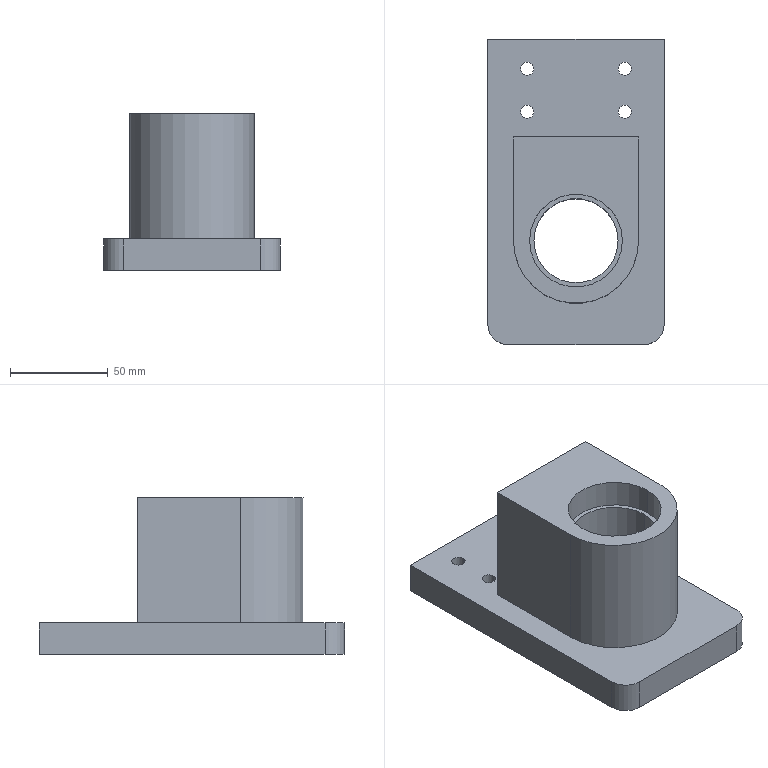Part | NX | 1 solid | 29 faces | box 90 x 156 x 80 mm | volume 416529 mm3 | cylinder 17 | plane 12 | commonest cylinder face diameters 6.8 x8 47.5 x4 20 x2 43 x2 64 x1
STEP:
#1=CARTESIAN_POINT('',(80.,0.,16.));
#2=VERTEX_POINT('',#1);
#3=CARTESIAN_POINT('',(90.,10.,16.));
#4=VERTEX_POINT('',#3);
#5=CARTESIAN_POINT('',(80.,10.,16.));
#6=DIRECTION('',(0.,0.,1.));
#7=DIRECTION('',(-1.,0.,0.));
#8=AXIS2_PLACEMENT_3D('',#5,#6,#7);
#9=CIRCLE('',#8,10.);
#10=EDGE_CURVE('',#2,#4,#9,.T.);
#11=ORIENTED_EDGE('',*,*,#10,.F.);
#12=CARTESIAN_POINT('',(80.,0.,0.));
#13=VERTEX_POINT('',#12);
#14=CARTESIAN_POINT('',(80.,0.,16.));
#15=DIRECTION('',(0.,0.,1.));
#16=VECTOR('',#15,1000.);
#17=LINE('',#14,#16);
#18=EDGE_CURVE('',#13,#2,#17,.T.);
#19=ORIENTED_EDGE('',*,*,#18,.F.);
#20=CARTESIAN_POINT('',(90.,10.,0.));
#21=VERTEX_POINT('',#20);
#22=CARTESIAN_POINT('',(80.,10.,0.));
#23=DIRECTION('',(0.,0.,-1.));
#24=DIRECTION('',(-1.,0.,0.));
#25=AXIS2_PLACEMENT_3D('',#22,#23,#24);
#26=CIRCLE('',#25,10.);
#27=EDGE_CURVE('',#21,#13,#26,.T.);
#28=ORIENTED_EDGE('',*,*,#27,.F.);
#29=CARTESIAN_POINT('',(90.,10.,16.));
#30=DIRECTION('',(0.,0.,-1.));
#31=VECTOR('',#30,1000.);
#32=LINE('',#29,#31);
#33=EDGE_CURVE('',#4,#21,#32,.T.);
#34=ORIENTED_EDGE('',*,*,#33,.F.);
#35=EDGE_LOOP('',(#11,#19,#28,#34));
#36=FACE_BOUND('',#35,.T.);
#37=CARTESIAN_POINT('',(80.,10.,16.));
#38=DIRECTION('',(0.,0.,-1.));
#39=DIRECTION('',(-1.,0.,0.));
#40=AXIS2_PLACEMENT_3D('',#37,#38,#39);
#41=CYLINDRICAL_SURFACE('',#40,10.);
#42=ADVANCED_FACE('',(#36),#41,.T.);
#43=CARTESIAN_POINT('',(0.,10.,16.));
#44=VERTEX_POINT('',#43);
#45=CARTESIAN_POINT('',(10.,0.,16.));
#46=VERTEX_POINT('',#45);
#47=CARTESIAN_POINT('',(10.,10.,16.));
#48=DIRECTION('',(0.,0.,1.));
#49=DIRECTION('',(-1.,0.,0.));
#50=AXIS2_PLACEMENT_3D('',#47,#48,#49);
#51=CIRCLE('',#50,10.);
#52=EDGE_CURVE('',#44,#46,#51,.T.);
#53=ORIENTED_EDGE('',*,*,#52,.F.);
#54=CARTESIAN_POINT('',(0.,10.,0.));
#55=VERTEX_POINT('',#54);
#56=CARTESIAN_POINT('',(0.,10.,16.));
#57=DIRECTION('',(0.,0.,1.));
#58=VECTOR('',#57,1000.);
#59=LINE('',#56,#58);
#60=EDGE_CURVE('',#55,#44,#59,.T.);
#61=ORIENTED_EDGE('',*,*,#60,.F.);
#62=CARTESIAN_POINT('',(10.,0.,0.));
#63=VERTEX_POINT('',#62);
#64=CARTESIAN_POINT('',(10.,10.,0.));
#65=DIRECTION('',(0.,0.,-1.));
#66=DIRECTION('',(-1.,0.,0.));
#67=AXIS2_PLACEMENT_3D('',#64,#65,#66);
#68=CIRCLE('',#67,10.);
#69=EDGE_CURVE('',#63,#55,#68,.T.);
#70=ORIENTED_EDGE('',*,*,#69,.F.);
#71=CARTESIAN_POINT('',(10.,0.,16.));
#72=DIRECTION('',(0.,0.,-1.));
#73=VECTOR('',#72,1000.);
#74=LINE('',#71,#73);
#75=EDGE_CURVE('',#46,#63,#74,.T.);
#76=ORIENTED_EDGE('',*,*,#75,.F.);
#77=EDGE_LOOP('',(#53,#61,#70,#76));
#78=FACE_BOUND('',#77,.T.);
#79=CARTESIAN_POINT('',(10.,10.,16.));
#80=DIRECTION('',(0.,0.,-1.));
#81=DIRECTION('',(-1.,0.,0.));
#82=AXIS2_PLACEMENT_3D('',#79,#80,#81);
#83=CYLINDRICAL_SURFACE('',#82,10.);
#84=ADVANCED_FACE('',(#78),#83,.T.);
#85=CARTESIAN_POINT('',(73.4,141.,16.));
#86=VERTEX_POINT('',#85);
#87=CARTESIAN_POINT('',(73.4,141.,0.));
#88=VERTEX_POINT('',#87);
#89=CARTESIAN_POINT('',(73.4,141.,0.));
#90=DIRECTION('',(0.,0.,-1.));
#91=VECTOR('',#90,1000.);
#92=LINE('',#89,#91);
#93=EDGE_CURVE('',#86,#88,#92,.T.);
#94=ORIENTED_EDGE('',*,*,#93,.F.);
#95=CARTESIAN_POINT('',(66.6,141.,16.));
#96=VERTEX_POINT('',#95);
#97=CARTESIAN_POINT('',(70.,141.,16.));
#98=DIRECTION('',(0.,0.,-1.));
#99=DIRECTION('',(-1.,0.,0.));
#100=AXIS2_PLACEMENT_3D('',#97,#98,#99);
#101=CIRCLE('',#100,3.4);
#102=EDGE_CURVE('',#96,#86,#101,.T.);
#103=ORIENTED_EDGE('',*,*,#102,.F.);
#104=CARTESIAN_POINT('',(66.6,141.,0.));
#105=VERTEX_POINT('',#104);
#106=CARTESIAN_POINT('',(66.6,141.,0.));
#107=DIRECTION('',(0.,0.,-1.));
#108=VECTOR('',#107,1000.);
#109=LINE('',#106,#108);
#110=EDGE_CURVE('',#96,#105,#109,.T.);
#111=ORIENTED_EDGE('',*,*,#110,.T.);
#112=CARTESIAN_POINT('',(70.,141.,0.));
#113=DIRECTION('',(0.,0.,-1.));
#114=DIRECTION('',(-1.,0.,0.));
#115=AXIS2_PLACEMENT_3D('',#112,#113,#114);
#116=CIRCLE('',#115,3.4);
#117=EDGE_CURVE('',#105,#88,#116,.T.);
#118=ORIENTED_EDGE('',*,*,#117,.T.);
#119=EDGE_LOOP('',(#94,#103,#111,#118));
#120=FACE_BOUND('',#119,.T.);
#121=CARTESIAN_POINT('',(70.,141.,0.));
#122=DIRECTION('',(0.,0.,-1.));
#123=DIRECTION('',(-1.,0.,0.));
#124=AXIS2_PLACEMENT_3D('',#121,#122,#123);
#125=CYLINDRICAL_SURFACE('',#124,3.4);
#126=ADVANCED_FACE('',(#120),#125,.F.);
#127=CARTESIAN_POINT('',(23.4,141.,16.));
#128=VERTEX_POINT('',#127);
#129=CARTESIAN_POINT('',(23.4,141.,0.));
#130=VERTEX_POINT('',#129);
#131=CARTESIAN_POINT('',(23.4,141.,0.));
#132=DIRECTION('',(0.,0.,-1.));
#133=VECTOR('',#132,1000.);
#134=LINE('',#131,#133);
#135=EDGE_CURVE('',#128,#130,#134,.T.);
#136=ORIENTED_EDGE('',*,*,#135,.F.);
#137=CARTESIAN_POINT('',(16.6,141.,16.));
#138=VERTEX_POINT('',#137);
#139=CARTESIAN_POINT('',(20.,141.,16.));
#140=DIRECTION('',(0.,0.,-1.));
#141=DIRECTION('',(-1.,0.,0.));
#142=AXIS2_PLACEMENT_3D('',#139,#140,#141);
#143=CIRCLE('',#142,3.4);
#144=EDGE_CURVE('',#138,#128,#143,.T.);
#145=ORIENTED_EDGE('',*,*,#144,.F.);
#146=CARTESIAN_POINT('',(16.6,141.,0.));
#147=VERTEX_POINT('',#146);
#148=CARTESIAN_POINT('',(16.6,141.,0.));
#149=DIRECTION('',(0.,0.,-1.));
#150=VECTOR('',#149,1000.);
#151=LINE('',#148,#150);
#152=EDGE_CURVE('',#138,#147,#151,.T.);
#153=ORIENTED_EDGE('',*,*,#152,.T.);
#154=CARTESIAN_POINT('',(20.,141.,0.));
#155=DIRECTION('',(0.,0.,-1.));
#156=DIRECTION('',(-1.,0.,0.));
#157=AXIS2_PLACEMENT_3D('',#154,#155,#156);
#158=CIRCLE('',#157,3.4);
#159=EDGE_CURVE('',#147,#130,#158,.T.);
#160=ORIENTED_EDGE('',*,*,#159,.T.);
#161=EDGE_LOOP('',(#136,#145,#153,#160));
#162=FACE_BOUND('',#161,.T.);
#163=CARTESIAN_POINT('',(20.,141.,0.));
#164=DIRECTION('',(0.,0.,-1.));
#165=DIRECTION('',(-1.,0.,0.));
#166=AXIS2_PLACEMENT_3D('',#163,#164,#165);
#167=CYLINDRICAL_SURFACE('',#166,3.4);
#168=ADVANCED_FACE('',(#162),#167,.F.);
#169=CARTESIAN_POINT('',(73.4,119.,16.));
#170=VERTEX_POINT('',#169);
#171=CARTESIAN_POINT('',(73.4,119.,0.));
#172=VERTEX_POINT('',#171);
#173=CARTESIAN_POINT('',(73.4,119.,0.));
#174=DIRECTION('',(0.,0.,-1.));
#175=VECTOR('',#174,1000.);
#176=LINE('',#173,#175);
#177=EDGE_CURVE('',#170,#172,#176,.T.);
#178=ORIENTED_EDGE('',*,*,#177,.F.);
#179=CARTESIAN_POINT('',(66.6,119.,16.));
#180=VERTEX_POINT('',#179);
#181=CARTESIAN_POINT('',(70.,119.,16.));
#182=DIRECTION('',(0.,0.,-1.));
#183=DIRECTION('',(-1.,0.,0.));
#184=AXIS2_PLACEMENT_3D('',#181,#182,#183);
#185=CIRCLE('',#184,3.4);
#186=EDGE_CURVE('',#180,#170,#185,.T.);
#187=ORIENTED_EDGE('',*,*,#186,.F.);
#188=CARTESIAN_POINT('',(66.6,119.,0.));
#189=VERTEX_POINT('',#188);
#190=CARTESIAN_POINT('',(66.6,119.,0.));
#191=DIRECTION('',(0.,0.,-1.));
#192=VECTOR('',#191,1000.);
#193=LINE('',#190,#192);
#194=EDGE_CURVE('',#180,#189,#193,.T.);
#195=ORIENTED_EDGE('',*,*,#194,.T.);
#196=CARTESIAN_POINT('',(70.,119.,0.));
#197=DIRECTION('',(0.,0.,-1.));
#198=DIRECTION('',(-1.,0.,0.));
#199=AXIS2_PLACEMENT_3D('',#196,#197,#198);
#200=CIRCLE('',#199,3.4);
#201=EDGE_CURVE('',#189,#172,#200,.T.);
#202=ORIENTED_EDGE('',*,*,#201,.T.);
#203=EDGE_LOOP('',(#178,#187,#195,#202));
#204=FACE_BOUND('',#203,.T.);
#205=CARTESIAN_POINT('',(70.,119.,0.));
#206=DIRECTION('',(0.,0.,-1.));
#207=DIRECTION('',(-1.,0.,0.));
#208=AXIS2_PLACEMENT_3D('',#205,#206,#207);
#209=CYLINDRICAL_SURFACE('',#208,3.4);
#210=ADVANCED_FACE('',(#204),#209,.F.);
#211=CARTESIAN_POINT('',(23.4,119.,16.));
#212=VERTEX_POINT('',#211);
#213=CARTESIAN_POINT('',(23.4,119.,0.));
#214=VERTEX_POINT('',#213);
#215=CARTESIAN_POINT('',(23.4,119.,0.));
#216=DIRECTION('',(0.,0.,-1.));
#217=VECTOR('',#216,1000.);
#218=LINE('',#215,#217);
#219=EDGE_CURVE('',#212,#214,#218,.T.);
#220=ORIENTED_EDGE('',*,*,#219,.F.);
#221=CARTESIAN_POINT('',(16.6,119.,16.));
#222=VERTEX_POINT('',#221);
#223=CARTESIAN_POINT('',(20.,119.,16.));
#224=DIRECTION('',(0.,0.,-1.));
#225=DIRECTION('',(-1.,0.,0.));
#226=AXIS2_PLACEMENT_3D('',#223,#224,#225);
#227=CIRCLE('',#226,3.4);
#228=EDGE_CURVE('',#222,#212,#227,.T.);
#229=ORIENTED_EDGE('',*,*,#228,.F.);
#230=CARTESIAN_POINT('',(16.6,119.,0.));
#231=VERTEX_POINT('',#230);
#232=CARTESIAN_POINT('',(16.6,119.,0.));
#233=DIRECTION('',(0.,0.,-1.));
#234=VECTOR('',#233,1000.);
#235=LINE('',#232,#234);
#236=EDGE_CURVE('',#222,#231,#235,.T.);
#237=ORIENTED_EDGE('',*,*,#236,.T.);
#238=CARTESIAN_POINT('',(20.,119.,0.));
#239=DIRECTION('',(0.,0.,-1.));
#240=DIRECTION('',(-1.,0.,0.));
#241=AXIS2_PLACEMENT_3D('',#238,#239,#240);
#242=CIRCLE('',#241,3.4);
#243=EDGE_CURVE('',#231,#214,#242,.T.);
#244=ORIENTED_EDGE('',*,*,#243,.T.);
#245=EDGE_LOOP('',(#220,#229,#237,#244));
#246=FACE_BOUND('',#245,.T.);
#247=CARTESIAN_POINT('',(20.,119.,0.));
#248=DIRECTION('',(0.,0.,-1.));
#249=DIRECTION('',(-1.,0.,0.));
#250=AXIS2_PLACEMENT_3D('',#247,#248,#249);
#251=CYLINDRICAL_SURFACE('',#250,3.4);
#252=ADVANCED_FACE('',(#246),#251,.F.);
#253=CARTESIAN_POINT('',(13.,106.,16.));
#254=VERTEX_POINT('',#253);
#255=CARTESIAN_POINT('',(13.,53.,16.));
#256=VERTEX_POINT('',#255);
#257=CARTESIAN_POINT('',(13.,53.,16.));
#258=DIRECTION('',(0.,-1.,0.));
#259=VECTOR('',#258,1000.);
#260=LINE('',#257,#259);
#261=EDGE_CURVE('',#254,#256,#260,.T.);
#262=ORIENTED_EDGE('',*,*,#261,.T.);
#263=CARTESIAN_POINT('',(13.,53.,80.));
#264=VERTEX_POINT('',#263);
#265=CARTESIAN_POINT('',(13.,53.,80.));
#266=DIRECTION('',(0.,0.,-1.));
#267=VECTOR('',#266,1000.);
#268=LINE('',#265,#267);
#269=EDGE_CURVE('',#264,#256,#268,.T.);
#270=ORIENTED_EDGE('',*,*,#269,.F.);
#271=CARTESIAN_POINT('',(13.,106.,80.));
#272=VERTEX_POINT('',#271);
#273=CARTESIAN_POINT('',(13.,53.,80.));
#274=DIRECTION('',(0.,-1.,0.));
#275=VECTOR('',#274,1000.);
#276=LINE('',#273,#275);
#277=EDGE_CURVE('',#272,#264,#276,.T.);
#278=ORIENTED_EDGE('',*,*,#277,.F.);
#279=CARTESIAN_POINT('',(13.,106.,80.));
#280=DIRECTION('',(0.,0.,-1.));
#281=VECTOR('',#280,1000.);
#282=LINE('',#279,#281);
#283=EDGE_CURVE('',#272,#254,#282,.T.);
#284=ORIENTED_EDGE('',*,*,#283,.T.);
#285=EDGE_LOOP('',(#262,#270,#278,#284));
#286=FACE_BOUND('',#285,.T.);
#287=CARTESIAN_POINT('',(13.,53.,80.));
#288=DIRECTION('',(1.,0.,0.));
#289=DIRECTION('',(0.,0.,-1.));
#290=AXIS2_PLACEMENT_3D('',#287,#288,#289);
#291=PLANE('',#290);
#292=ADVANCED_FACE('',(#286),#291,.F.);
#293=CARTESIAN_POINT('',(77.,106.,16.));
#294=VERTEX_POINT('',#293);
#295=CARTESIAN_POINT('',(13.,106.,16.));
#296=DIRECTION('',(-1.,0.,0.));
#297=VECTOR('',#296,1000.);
#298=LINE('',#295,#297);
#299=EDGE_CURVE('',#294,#254,#298,.T.);
#300=ORIENTED_EDGE('',*,*,#299,.T.);
#301=ORIENTED_EDGE('',*,*,#283,.F.);
#302=CARTESIAN_POINT('',(77.,106.,80.));
#303=VERTEX_POINT('',#302);
#304=CARTESIAN_POINT('',(13.,106.,80.));
#305=DIRECTION('',(-1.,0.,0.));
#306=VECTOR('',#305,1000.);
#307=LINE('',#304,#306);
#308=EDGE_CURVE('',#303,#272,#307,.T.);
#309=ORIENTED_EDGE('',*,*,#308,.F.);
#310=CARTESIAN_POINT('',(77.,106.,80.));
#311=DIRECTION('',(0.,0.,-1.));
#312=VECTOR('',#311,1000.);
#313=LINE('',#310,#312);
#314=EDGE_CURVE('',#303,#294,#313,.T.);
#315=ORIENTED_EDGE('',*,*,#314,.T.);
#316=EDGE_LOOP('',(#300,#301,#309,#315));
#317=FACE_BOUND('',#316,.T.);
#318=CARTESIAN_POINT('',(13.,106.,80.));
#319=DIRECTION('',(0.,-1.,0.));
#320=DIRECTION('',(0.,0.,-1.));
#321=AXIS2_PLACEMENT_3D('',#318,#319,#320);
#322=PLANE('',#321);
#323=ADVANCED_FACE('',(#317),#322,.F.);
#324=CARTESIAN_POINT('',(77.,53.,16.));
#325=VERTEX_POINT('',#324);
#326=CARTESIAN_POINT('',(77.,106.,16.));
#327=DIRECTION('',(0.,1.,0.));
#328=VECTOR('',#327,1000.);
#329=LINE('',#326,#328);
#330=EDGE_CURVE('',#325,#294,#329,.T.);
#331=ORIENTED_EDGE('',*,*,#330,.T.);
#332=ORIENTED_EDGE('',*,*,#314,.F.);
#333=CARTESIAN_POINT('',(77.,53.,80.));
#334=VERTEX_POINT('',#333);
#335=CARTESIAN_POINT('',(77.,106.,80.));
#336=DIRECTION('',(0.,1.,0.));
#337=VECTOR('',#336,1000.);
#338=LINE('',#335,#337);
#339=EDGE_CURVE('',#334,#303,#338,.T.);
#340=ORIENTED_EDGE('',*,*,#339,.F.);
#341=CARTESIAN_POINT('',(77.,53.,80.));
#342=DIRECTION('',(0.,0.,-1.));
#343=VECTOR('',#342,1000.);
#344=LINE('',#341,#343);
#345=EDGE_CURVE('',#334,#325,#344,.T.);
#346=ORIENTED_EDGE('',*,*,#345,.T.);
#347=EDGE_LOOP('',(#331,#332,#340,#346));
#348=FACE_BOUND('',#347,.T.);
#349=CARTESIAN_POINT('',(77.,106.,80.));
#350=DIRECTION('',(-1.,0.,0.));
#351=DIRECTION('',(0.,0.,1.));
#352=AXIS2_PLACEMENT_3D('',#349,#350,#351);
#353=PLANE('',#352);
#354=ADVANCED_FACE('',(#348),#353,.F.);
#355=CARTESIAN_POINT('',(68.75,53.,14.));
#356=VERTEX_POINT('',#355);
#357=CARTESIAN_POINT('',(68.75,53.,0.));
#358=VERTEX_POINT('',#357);
#359=CARTESIAN_POINT('',(68.75,53.,14.));
#360=DIRECTION('',(0.,0.,-1.));
#361=VECTOR('',#360,1000.);
#362=LINE('',#359,#361);
#363=EDGE_CURVE('',#356,#358,#362,.T.);
#364=ORIENTED_EDGE('',*,*,#363,.F.);
#365=CARTESIAN_POINT('',(21.25,53.,14.));
#366=VERTEX_POINT('',#365);
#367=CARTESIAN_POINT('',(45.,53.,14.));
#368=DIRECTION('',(0.,0.,-1.));
#369=DIRECTION('',(-1.,0.,0.));
#370=AXIS2_PLACEMENT_3D('',#367,#368,#369);
#371=CIRCLE('',#370,23.75);
#372=EDGE_CURVE('',#366,#356,#371,.T.);
#373=ORIENTED_EDGE('',*,*,#372,.F.);
#374=CARTESIAN_POINT('',(21.25,53.,0.));
#375=VERTEX_POINT('',#374);
#376=CARTESIAN_POINT('',(21.25,53.,14.));
#377=DIRECTION('',(0.,0.,-1.));
#378=VECTOR('',#377,1000.);
#379=LINE('',#376,#378);
#380=EDGE_CURVE('',#366,#375,#379,.T.);
#381=ORIENTED_EDGE('',*,*,#380,.T.);
#382=CARTESIAN_POINT('',(45.,53.,0.));
#383=DIRECTION('',(0.,0.,-1.));
#384=DIRECTION('',(-1.,0.,0.));
#385=AXIS2_PLACEMENT_3D('',#382,#383,#384);
#386=CIRCLE('',#385,23.75);
#387=EDGE_CURVE('',#375,#358,#386,.T.);
#388=ORIENTED_EDGE('',*,*,#387,.T.);
#389=EDGE_LOOP('',(#364,#373,#381,#388));
#390=FACE_BOUND('',#389,.T.);
#391=CARTESIAN_POINT('',(45.,53.,14.));
#392=DIRECTION('',(0.,0.,-1.));
#393=DIRECTION('',(-1.,0.,0.));
#394=AXIS2_PLACEMENT_3D('',#391,#392,#393);
#395=CYLINDRICAL_SURFACE('',#394,23.75);
#396=ADVANCED_FACE('',(#390),#395,.F.);
#397=CARTESIAN_POINT('',(66.5,53.,14.));
#398=VERTEX_POINT('',#397);
#399=CARTESIAN_POINT('',(23.5,53.,14.));
#400=VERTEX_POINT('',#399);
#401=CARTESIAN_POINT('',(45.,53.,14.));
#402=DIRECTION('',(0.,0.,1.));
#403=DIRECTION('',(-1.,0.,0.));
#404=AXIS2_PLACEMENT_3D('',#401,#402,#403);
#405=CIRCLE('',#404,21.5);
#406=EDGE_CURVE('',#398,#400,#405,.T.);
#407=ORIENTED_EDGE('',*,*,#406,.T.);
#408=CARTESIAN_POINT('',(45.,53.,14.));
#409=DIRECTION('',(0.,0.,1.));
#410=DIRECTION('',(-1.,0.,0.));
#411=AXIS2_PLACEMENT_3D('',#408,#409,#410);
#412=CIRCLE('',#411,21.5);
#413=EDGE_CURVE('',#400,#398,#412,.T.);
#414=ORIENTED_EDGE('',*,*,#413,.T.);
#415=EDGE_LOOP('',(#407,#414));
#416=FACE_BOUND('',#415,.T.);
#417=ORIENTED_EDGE('',*,*,#372,.T.);
#418=CARTESIAN_POINT('',(45.,53.,14.));
#419=DIRECTION('',(0.,0.,-1.));
#420=DIRECTION('',(-1.,0.,0.));
#421=AXIS2_PLACEMENT_3D('',#418,#419,#420);
#422=CIRCLE('',#421,23.75);
#423=EDGE_CURVE('',#356,#366,#422,.T.);
#424=ORIENTED_EDGE('',*,*,#423,.T.);
#425=EDGE_LOOP('',(#417,#424));
#426=FACE_BOUND('',#425,.T.);
#427=CARTESIAN_POINT('',(45.,53.,14.));
#428=DIRECTION('',(0.,0.,-1.));
#429=DIRECTION('',(-1.,0.,0.));
#430=AXIS2_PLACEMENT_3D('',#427,#428,#429);
#431=PLANE('',#430);
#432=ADVANCED_FACE('',(#416,#426),#431,.T.);
#433=CARTESIAN_POINT('',(21.25,53.,66.));
#434=VERTEX_POINT('',#433);
#435=CARTESIAN_POINT('',(21.25,53.,80.));
#436=VERTEX_POINT('',#435);
#437=CARTESIAN_POINT('',(21.25,53.,66.));
#438=DIRECTION('',(0.,0.,1.));
#439=VECTOR('',#438,1000.);
#440=LINE('',#437,#439);
#441=EDGE_CURVE('',#434,#436,#440,.T.);
#442=ORIENTED_EDGE('',*,*,#441,.F.);
#443=CARTESIAN_POINT('',(68.75,53.,66.));
#444=VERTEX_POINT('',#443);
#445=CARTESIAN_POINT('',(45.,53.,66.));
#446=DIRECTION('',(0.,0.,1.));
#447=DIRECTION('',(1.,0.,0.));
#448=AXIS2_PLACEMENT_3D('',#445,#446,#447);
#449=CIRCLE('',#448,23.75);
#450=EDGE_CURVE('',#444,#434,#449,.T.);
#451=ORIENTED_EDGE('',*,*,#450,.F.);
#452=CARTESIAN_POINT('',(68.75,53.,80.));
#453=VERTEX_POINT('',#452);
#454=CARTESIAN_POINT('',(68.75,53.,66.));
#455=DIRECTION('',(0.,0.,1.));
#456=VECTOR('',#455,1000.);
#457=LINE('',#454,#456);
#458=EDGE_CURVE('',#444,#453,#457,.T.);
#459=ORIENTED_EDGE('',*,*,#458,.T.);
#460=CARTESIAN_POINT('',(45.,53.,80.));
#461=DIRECTION('',(0.,0.,1.));
#462=DIRECTION('',(1.,0.,0.));
#463=AXIS2_PLACEMENT_3D('',#460,#461,#462);
#464=CIRCLE('',#463,23.75);
#465=EDGE_CURVE('',#453,#436,#464,.T.);
#466=ORIENTED_EDGE('',*,*,#465,.T.);
#467=EDGE_LOOP('',(#442,#451,#459,#466));
#468=FACE_BOUND('',#467,.T.);
#469=CARTESIAN_POINT('',(45.,53.,66.));
#470=DIRECTION('',(0.,0.,1.));
#471=DIRECTION('',(1.,0.,0.));
#472=AXIS2_PLACEMENT_3D('',#469,#470,#471);
#473=CYLINDRICAL_SURFACE('',#472,23.75);
#474=ADVANCED_FACE('',(#468),#473,.F.);
#475=CARTESIAN_POINT('',(66.5,53.,66.));
#476=VERTEX_POINT('',#475);
#477=CARTESIAN_POINT('',(23.5,53.,66.));
#478=VERTEX_POINT('',#477);
#479=CARTESIAN_POINT('',(45.,53.,66.));
#480=DIRECTION('',(0.,0.,-1.));
#481=DIRECTION('',(1.,0.,0.));
#482=AXIS2_PLACEMENT_3D('',#479,#480,#481);
#483=CIRCLE('',#482,21.5);
#484=EDGE_CURVE('',#476,#478,#483,.T.);
#485=ORIENTED_EDGE('',*,*,#484,.T.);
#486=CARTESIAN_POINT('',(45.,53.,66.));
#487=DIRECTION('',(0.,0.,-1.));
#488=DIRECTION('',(1.,0.,0.));
#489=AXIS2_PLACEMENT_3D('',#486,#487,#488);
#490=CIRCLE('',#489,21.5);
#491=EDGE_CURVE('',#478,#476,#490,.T.);
#492=ORIENTED_EDGE('',*,*,#491,.T.);
#493=EDGE_LOOP('',(#485,#492));
#494=FACE_BOUND('',#493,.T.);
#495=ORIENTED_EDGE('',*,*,#450,.T.);
#496=CARTESIAN_POINT('',(45.,53.,66.));
#497=DIRECTION('',(0.,0.,1.));
#498=DIRECTION('',(1.,0.,0.));
#499=AXIS2_PLACEMENT_3D('',#496,#497,#498);
#500=CIRCLE('',#499,23.75);
#501=EDGE_CURVE('',#434,#444,#500,.T.);
#502=ORIENTED_EDGE('',*,*,#501,.T.);
#503=EDGE_LOOP('',(#495,#502));
#504=FACE_BOUND('',#503,.T.);
#505=CARTESIAN_POINT('',(45.,53.,66.));
#506=DIRECTION('',(0.,0.,1.));
#507=DIRECTION('',(1.,0.,0.));
#508=AXIS2_PLACEMENT_3D('',#505,#506,#507);
#509=PLANE('',#508);
#510=ADVANCED_FACE('',(#494,#504),#509,.T.);
#511=CARTESIAN_POINT('',(45.,53.,80.));
#512=DIRECTION('',(0.,0.,1.));
#513=DIRECTION('',(1.,0.,0.));
#514=AXIS2_PLACEMENT_3D('',#511,#512,#513);
#515=CIRCLE('',#514,32.);
#516=EDGE_CURVE('',#264,#334,#515,.T.);
#517=ORIENTED_EDGE('',*,*,#516,.T.);
#518=ORIENTED_EDGE('',*,*,#339,.T.);
#519=ORIENTED_EDGE('',*,*,#308,.T.);
#520=ORIENTED_EDGE('',*,*,#277,.T.);
#521=EDGE_LOOP('',(#517,#518,#519,#520));
#522=FACE_BOUND('',#521,.T.);
#523=ORIENTED_EDGE('',*,*,#465,.F.);
#524=CARTESIAN_POINT('',(45.,53.,80.));
#525=DIRECTION('',(0.,0.,1.));
#526=DIRECTION('',(1.,0.,0.));
#527=AXIS2_PLACEMENT_3D('',#524,#525,#526);
#528=CIRCLE('',#527,23.75);
#529=EDGE_CURVE('',#436,#453,#528,.T.);
#530=ORIENTED_EDGE('',*,*,#529,.F.);
#531=EDGE_LOOP('',(#523,#530));
#532=FACE_BOUND('',#531,.T.);
#533=CARTESIAN_POINT('',(45.,53.,80.));
#534=DIRECTION('',(0.,0.,1.));
#535=DIRECTION('',(1.,0.,0.));
#536=AXIS2_PLACEMENT_3D('',#533,#534,#535);
#537=PLANE('',#536);
#538=ADVANCED_FACE('',(#522,#532),#537,.T.);
#539=CARTESIAN_POINT('',(0.,0.,0.));
#540=DIRECTION('',(1.,0.,0.));
#541=VECTOR('',#540,1000.);
#542=LINE('',#539,#541);
#543=EDGE_CURVE('',#63,#13,#542,.T.);
#544=ORIENTED_EDGE('',*,*,#543,.F.);
#545=ORIENTED_EDGE('',*,*,#69,.T.);
#546=CARTESIAN_POINT('',(0.,156.,0.));
#547=VERTEX_POINT('',#546);
#548=CARTESIAN_POINT('',(0.,0.,0.));
#549=DIRECTION('',(0.,-1.,0.));
#550=VECTOR('',#549,1000.);
#551=LINE('',#548,#550);
#552=EDGE_CURVE('',#547,#55,#551,.T.);
#553=ORIENTED_EDGE('',*,*,#552,.F.);
#554=CARTESIAN_POINT('',(90.,156.,0.));
#555=VERTEX_POINT('',#554);
#556=CARTESIAN_POINT('',(0.,156.,0.));
#557=DIRECTION('',(-1.,0.,0.));
#558=VECTOR('',#557,1000.);
#559=LINE('',#556,#558);
#560=EDGE_CURVE('',#555,#547,#559,.T.);
#561=ORIENTED_EDGE('',*,*,#560,.F.);
#562=CARTESIAN_POINT('',(90.,0.,0.));
#563=DIRECTION('',(0.,1.,0.));
#564=VECTOR('',#563,1000.);
#565=LINE('',#562,#564);
#566=EDGE_CURVE('',#21,#555,#565,.T.);
#567=ORIENTED_EDGE('',*,*,#566,.F.);
#568=ORIENTED_EDGE('',*,*,#27,.T.);
#569=EDGE_LOOP('',(#544,#545,#553,#561,#567,#568));
#570=FACE_BOUND('',#569,.T.);
#571=ORIENTED_EDGE('',*,*,#387,.F.);
#572=CARTESIAN_POINT('',(45.,53.,0.));
#573=DIRECTION('',(0.,0.,-1.));
#574=DIRECTION('',(-1.,0.,0.));
#575=AXIS2_PLACEMENT_3D('',#572,#573,#574);
#576=CIRCLE('',#575,23.75);
#577=EDGE_CURVE('',#358,#375,#576,.T.);
#578=ORIENTED_EDGE('',*,*,#577,.F.);
#579=EDGE_LOOP('',(#571,#578));
#580=FACE_BOUND('',#579,.T.);
#581=ORIENTED_EDGE('',*,*,#243,.F.);
#582=CARTESIAN_POINT('',(20.,119.,0.));
#583=DIRECTION('',(0.,0.,-1.));
#584=DIRECTION('',(-1.,0.,0.));
#585=AXIS2_PLACEMENT_3D('',#582,#583,#584);
#586=CIRCLE('',#585,3.4);
#587=EDGE_CURVE('',#214,#231,#586,.T.);
#588=ORIENTED_EDGE('',*,*,#587,.F.);
#589=EDGE_LOOP('',(#581,#588));
#590=FACE_BOUND('',#589,.T.);
#591=ORIENTED_EDGE('',*,*,#201,.F.);
#592=CARTESIAN_POINT('',(70.,119.,0.));
#593=DIRECTION('',(0.,0.,-1.));
#594=DIRECTION('',(-1.,0.,0.));
#595=AXIS2_PLACEMENT_3D('',#592,#593,#594);
#596=CIRCLE('',#595,3.4);
#597=EDGE_CURVE('',#172,#189,#596,.T.);
#598=ORIENTED_EDGE('',*,*,#597,.F.);
#599=EDGE_LOOP('',(#591,#598));
#600=FACE_BOUND('',#599,.T.);
#601=ORIENTED_EDGE('',*,*,#159,.F.);
#602=CARTESIAN_POINT('',(20.,141.,0.));
#603=DIRECTION('',(0.,0.,-1.));
#604=DIRECTION('',(-1.,0.,0.));
#605=AXIS2_PLACEMENT_3D('',#602,#603,#604);
#606=CIRCLE('',#605,3.4);
#607=EDGE_CURVE('',#130,#147,#606,.T.);
#608=ORIENTED_EDGE('',*,*,#607,.F.);
#609=EDGE_LOOP('',(#601,#608));
#610=FACE_BOUND('',#609,.T.);
#611=ORIENTED_EDGE('',*,*,#117,.F.);
#612=CARTESIAN_POINT('',(70.,141.,0.));
#613=DIRECTION('',(0.,0.,-1.));
#614=DIRECTION('',(-1.,0.,0.));
#615=AXIS2_PLACEMENT_3D('',#612,#613,#614);
#616=CIRCLE('',#615,3.4);
#617=EDGE_CURVE('',#88,#105,#616,.T.);
#618=ORIENTED_EDGE('',*,*,#617,.F.);
#619=EDGE_LOOP('',(#611,#618));
#620=FACE_BOUND('',#619,.T.);
#621=CARTESIAN_POINT('',(0.,0.,0.));
#622=DIRECTION('',(0.,0.,-1.));
#623=DIRECTION('',(-1.,0.,0.));
#624=AXIS2_PLACEMENT_3D('',#621,#622,#623);
#625=PLANE('',#624);
#626=ADVANCED_FACE('',(#570,#580,#590,#600,#610,#620),#625,.T.);
#627=ORIENTED_EDGE('',*,*,#560,.T.);
#628=CARTESIAN_POINT('',(0.,156.,16.));
#629=VERTEX_POINT('',#628);
#630=CARTESIAN_POINT('',(0.,156.,16.));
#631=DIRECTION('',(0.,0.,-1.));
#632=VECTOR('',#631,1000.);
#633=LINE('',#630,#632);
#634=EDGE_CURVE('',#629,#547,#633,.T.);
#635=ORIENTED_EDGE('',*,*,#634,.F.);
#636=CARTESIAN_POINT('',(90.,156.,16.));
#637=VERTEX_POINT('',#636);
#638=CARTESIAN_POINT('',(0.,156.,16.));
#639=DIRECTION('',(-1.,0.,0.));
#640=VECTOR('',#639,1000.);
#641=LINE('',#638,#640);
#642=EDGE_CURVE('',#637,#629,#641,.T.);
#643=ORIENTED_EDGE('',*,*,#642,.F.);
#644=CARTESIAN_POINT('',(90.,156.,16.));
#645=DIRECTION('',(0.,0.,-1.));
#646=VECTOR('',#645,1000.);
#647=LINE('',#644,#646);
#648=EDGE_CURVE('',#637,#555,#647,.T.);
#649=ORIENTED_EDGE('',*,*,#648,.T.);
#650=EDGE_LOOP('',(#627,#635,#643,#649));
#651=FACE_BOUND('',#650,.T.);
#652=CARTESIAN_POINT('',(0.,156.,16.));
#653=DIRECTION('',(0.,-1.,0.));
#654=DIRECTION('',(0.,0.,-1.));
#655=AXIS2_PLACEMENT_3D('',#652,#653,#654);
#656=PLANE('',#655);
#657=ADVANCED_FACE('',(#651),#656,.F.);
#658=CARTESIAN_POINT('',(90.,0.,16.));
#659=DIRECTION('',(0.,1.,0.));
#660=VECTOR('',#659,1000.);
#661=LINE('',#658,#660);
#662=EDGE_CURVE('',#4,#637,#661,.T.);
#663=ORIENTED_EDGE('',*,*,#662,.F.);
#664=ORIENTED_EDGE('',*,*,#33,.T.);
#665=ORIENTED_EDGE('',*,*,#566,.T.);
#666=ORIENTED_EDGE('',*,*,#648,.F.);
#667=EDGE_LOOP('',(#663,#664,#665,#666));
#668=FACE_BOUND('',#667,.T.);
#669=CARTESIAN_POINT('',(90.,0.,16.));
#670=DIRECTION('',(-1.,0.,0.));
#671=DIRECTION('',(0.,0.,1.));
#672=AXIS2_PLACEMENT_3D('',#669,#670,#671);
#673=PLANE('',#672);
#674=ADVANCED_FACE('',(#668),#673,.F.);
#675=CARTESIAN_POINT('',(0.,0.,16.));
#676=DIRECTION('',(1.,0.,0.));
#677=VECTOR('',#676,1000.);
#678=LINE('',#675,#677);
#679=EDGE_CURVE('',#46,#2,#678,.T.);
#680=ORIENTED_EDGE('',*,*,#679,.F.);
#681=ORIENTED_EDGE('',*,*,#75,.T.);
#682=ORIENTED_EDGE('',*,*,#543,.T.);
#683=ORIENTED_EDGE('',*,*,#18,.T.);
#684=EDGE_LOOP('',(#680,#681,#682,#683));
#685=FACE_BOUND('',#684,.T.);
#686=CARTESIAN_POINT('',(0.,0.,16.));
#687=DIRECTION('',(0.,1.,0.));
#688=DIRECTION('',(0.,0.,1.));
#689=AXIS2_PLACEMENT_3D('',#686,#687,#688);
#690=PLANE('',#689);
#691=ADVANCED_FACE('',(#685),#690,.F.);
#692=ORIENTED_EDGE('',*,*,#552,.T.);
#693=ORIENTED_EDGE('',*,*,#60,.T.);
#694=CARTESIAN_POINT('',(0.,0.,16.));
#695=DIRECTION('',(0.,-1.,0.));
#696=VECTOR('',#695,1000.);
#697=LINE('',#694,#696);
#698=EDGE_CURVE('',#629,#44,#697,.T.);
#699=ORIENTED_EDGE('',*,*,#698,.F.);
#700=ORIENTED_EDGE('',*,*,#634,.T.);
#701=EDGE_LOOP('',(#692,#693,#699,#700));
#702=FACE_BOUND('',#701,.T.);
#703=CARTESIAN_POINT('',(0.,0.,16.));
#704=DIRECTION('',(1.,0.,0.));
#705=DIRECTION('',(0.,0.,-1.));
#706=AXIS2_PLACEMENT_3D('',#703,#704,#705);
#707=PLANE('',#706);
#708=ADVANCED_FACE('',(#702),#707,.F.);
#709=CARTESIAN_POINT('',(23.5,53.,0.));
#710=DIRECTION('',(0.,0.,1.));
#711=VECTOR('',#710,1000.);
#712=LINE('',#709,#711);
#713=EDGE_CURVE('',#400,#478,#712,.T.);
#714=ORIENTED_EDGE('',*,*,#713,.F.);
#715=ORIENTED_EDGE('',*,*,#406,.F.);
#716=CARTESIAN_POINT('',(66.5,53.,0.));
#717=DIRECTION('',(0.,0.,1.));
#718=VECTOR('',#717,1000.);
#719=LINE('',#716,#718);
#720=EDGE_CURVE('',#398,#476,#719,.T.);
#721=ORIENTED_EDGE('',*,*,#720,.T.);
#722=ORIENTED_EDGE('',*,*,#491,.F.);
#723=EDGE_LOOP('',(#714,#715,#721,#722));
#724=FACE_BOUND('',#723,.T.);
#725=CARTESIAN_POINT('',(45.,53.,0.));
#726=DIRECTION('',(0.,0.,1.));
#727=DIRECTION('',(1.,0.,0.));
#728=AXIS2_PLACEMENT_3D('',#725,#726,#727);
#729=CYLINDRICAL_SURFACE('',#728,21.5);
#730=ADVANCED_FACE('',(#724),#729,.F.);
#731=ORIENTED_EDGE('',*,*,#345,.F.);
#732=ORIENTED_EDGE('',*,*,#516,.F.);
#733=ORIENTED_EDGE('',*,*,#269,.T.);
#734=CARTESIAN_POINT('',(45.,53.,16.));
#735=DIRECTION('',(0.,0.,1.));
#736=DIRECTION('',(-1.,0.,0.));
#737=AXIS2_PLACEMENT_3D('',#734,#735,#736);
#738=CIRCLE('',#737,32.);
#739=EDGE_CURVE('',#256,#325,#738,.T.);
#740=ORIENTED_EDGE('',*,*,#739,.T.);
#741=EDGE_LOOP('',(#731,#732,#733,#740));
#742=FACE_BOUND('',#741,.T.);
#743=CARTESIAN_POINT('',(45.,53.,80.));
#744=DIRECTION('',(0.,0.,-1.));
#745=DIRECTION('',(-1.,0.,0.));
#746=AXIS2_PLACEMENT_3D('',#743,#744,#745);
#747=CYLINDRICAL_SURFACE('',#746,32.);
#748=ADVANCED_FACE('',(#742),#747,.T.);
#749=ORIENTED_EDGE('',*,*,#330,.F.);
#750=ORIENTED_EDGE('',*,*,#739,.F.);
#751=ORIENTED_EDGE('',*,*,#261,.F.);
#752=ORIENTED_EDGE('',*,*,#299,.F.);
#753=EDGE_LOOP('',(#749,#750,#751,#752));
#754=FACE_BOUND('',#753,.T.);
#755=ORIENTED_EDGE('',*,*,#698,.T.);
#756=ORIENTED_EDGE('',*,*,#52,.T.);
#757=ORIENTED_EDGE('',*,*,#679,.T.);
#758=ORIENTED_EDGE('',*,*,#10,.T.);
#759=ORIENTED_EDGE('',*,*,#662,.T.);
#760=ORIENTED_EDGE('',*,*,#642,.T.);
#761=EDGE_LOOP('',(#755,#756,#757,#758,#759,#760));
#762=FACE_BOUND('',#761,.T.);
#763=ORIENTED_EDGE('',*,*,#228,.T.);
#764=CARTESIAN_POINT('',(20.,119.,16.));
#765=DIRECTION('',(0.,0.,-1.));
#766=DIRECTION('',(-1.,0.,0.));
#767=AXIS2_PLACEMENT_3D('',#764,#765,#766);
#768=CIRCLE('',#767,3.4);
#769=EDGE_CURVE('',#212,#222,#768,.T.);
#770=ORIENTED_EDGE('',*,*,#769,.T.);
#771=EDGE_LOOP('',(#763,#770));
#772=FACE_BOUND('',#771,.T.);
#773=ORIENTED_EDGE('',*,*,#186,.T.);
#774=CARTESIAN_POINT('',(70.,119.,16.));
#775=DIRECTION('',(0.,0.,-1.));
#776=DIRECTION('',(-1.,0.,0.));
#777=AXIS2_PLACEMENT_3D('',#774,#775,#776);
#778=CIRCLE('',#777,3.4);
#779=EDGE_CURVE('',#170,#180,#778,.T.);
#780=ORIENTED_EDGE('',*,*,#779,.T.);
#781=EDGE_LOOP('',(#773,#780));
#782=FACE_BOUND('',#781,.T.);
#783=ORIENTED_EDGE('',*,*,#144,.T.);
#784=CARTESIAN_POINT('',(20.,141.,16.));
#785=DIRECTION('',(0.,0.,-1.));
#786=DIRECTION('',(-1.,0.,0.));
#787=AXIS2_PLACEMENT_3D('',#784,#785,#786);
#788=CIRCLE('',#787,3.4);
#789=EDGE_CURVE('',#128,#138,#788,.T.);
#790=ORIENTED_EDGE('',*,*,#789,.T.);
#791=EDGE_LOOP('',(#783,#790));
#792=FACE_BOUND('',#791,.T.);
#793=ORIENTED_EDGE('',*,*,#102,.T.);
#794=CARTESIAN_POINT('',(70.,141.,16.));
#795=DIRECTION('',(0.,0.,-1.));
#796=DIRECTION('',(-1.,0.,0.));
#797=AXIS2_PLACEMENT_3D('',#794,#795,#796);
#798=CIRCLE('',#797,3.4);
#799=EDGE_CURVE('',#86,#96,#798,.T.);
#800=ORIENTED_EDGE('',*,*,#799,.T.);
#801=EDGE_LOOP('',(#793,#800));
#802=FACE_BOUND('',#801,.T.);
#803=CARTESIAN_POINT('',(0.,0.,16.));
#804=DIRECTION('',(0.,0.,-1.));
#805=DIRECTION('',(-1.,0.,0.));
#806=AXIS2_PLACEMENT_3D('',#803,#804,#805);
#807=PLANE('',#806);
#808=ADVANCED_FACE('',(#754,#762,#772,#782,#792,#802),#807,.F.);
#809=ORIENTED_EDGE('',*,*,#413,.F.);
#810=ORIENTED_EDGE('',*,*,#713,.T.);
#811=ORIENTED_EDGE('',*,*,#484,.F.);
#812=ORIENTED_EDGE('',*,*,#720,.F.);
#813=EDGE_LOOP('',(#809,#810,#811,#812));
#814=FACE_BOUND('',#813,.T.);
#815=CARTESIAN_POINT('',(45.,53.,0.));
#816=DIRECTION('',(0.,0.,1.));
#817=DIRECTION('',(1.,0.,0.));
#818=AXIS2_PLACEMENT_3D('',#815,#816,#817);
#819=CYLINDRICAL_SURFACE('',#818,21.5);
#820=ADVANCED_FACE('',(#814),#819,.F.);
#821=ORIENTED_EDGE('',*,*,#501,.F.);
#822=ORIENTED_EDGE('',*,*,#441,.T.);
#823=ORIENTED_EDGE('',*,*,#529,.T.);
#824=ORIENTED_EDGE('',*,*,#458,.F.);
#825=EDGE_LOOP('',(#821,#822,#823,#824));
#826=FACE_BOUND('',#825,.T.);
#827=CARTESIAN_POINT('',(45.,53.,66.));
#828=DIRECTION('',(0.,0.,1.));
#829=DIRECTION('',(1.,0.,0.));
#830=AXIS2_PLACEMENT_3D('',#827,#828,#829);
#831=CYLINDRICAL_SURFACE('',#830,23.75);
#832=ADVANCED_FACE('',(#826),#831,.F.);
#833=ORIENTED_EDGE('',*,*,#423,.F.);
#834=ORIENTED_EDGE('',*,*,#363,.T.);
#835=ORIENTED_EDGE('',*,*,#577,.T.);
#836=ORIENTED_EDGE('',*,*,#380,.F.);
#837=EDGE_LOOP('',(#833,#834,#835,#836));
#838=FACE_BOUND('',#837,.T.);
#839=CARTESIAN_POINT('',(45.,53.,14.));
#840=DIRECTION('',(0.,0.,-1.));
#841=DIRECTION('',(-1.,0.,0.));
#842=AXIS2_PLACEMENT_3D('',#839,#840,#841);
#843=CYLINDRICAL_SURFACE('',#842,23.75);
#844=ADVANCED_FACE('',(#838),#843,.F.);
#845=ORIENTED_EDGE('',*,*,#769,.F.);
#846=ORIENTED_EDGE('',*,*,#219,.T.);
#847=ORIENTED_EDGE('',*,*,#587,.T.);
#848=ORIENTED_EDGE('',*,*,#236,.F.);
#849=EDGE_LOOP('',(#845,#846,#847,#848));
#850=FACE_BOUND('',#849,.T.);
#851=CARTESIAN_POINT('',(20.,119.,0.));
#852=DIRECTION('',(0.,0.,-1.));
#853=DIRECTION('',(-1.,0.,0.));
#854=AXIS2_PLACEMENT_3D('',#851,#852,#853);
#855=CYLINDRICAL_SURFACE('',#854,3.4);
#856=ADVANCED_FACE('',(#850),#855,.F.);
#857=ORIENTED_EDGE('',*,*,#779,.F.);
#858=ORIENTED_EDGE('',*,*,#177,.T.);
#859=ORIENTED_EDGE('',*,*,#597,.T.);
#860=ORIENTED_EDGE('',*,*,#194,.F.);
#861=EDGE_LOOP('',(#857,#858,#859,#860));
#862=FACE_BOUND('',#861,.T.);
#863=CARTESIAN_POINT('',(70.,119.,0.));
#864=DIRECTION('',(0.,0.,-1.));
#865=DIRECTION('',(-1.,0.,0.));
#866=AXIS2_PLACEMENT_3D('',#863,#864,#865);
#867=CYLINDRICAL_SURFACE('',#866,3.4);
#868=ADVANCED_FACE('',(#862),#867,.F.);
#869=ORIENTED_EDGE('',*,*,#789,.F.);
#870=ORIENTED_EDGE('',*,*,#135,.T.);
#871=ORIENTED_EDGE('',*,*,#607,.T.);
#872=ORIENTED_EDGE('',*,*,#152,.F.);
#873=EDGE_LOOP('',(#869,#870,#871,#872));
#874=FACE_BOUND('',#873,.T.);
#875=CARTESIAN_POINT('',(20.,141.,0.));
#876=DIRECTION('',(0.,0.,-1.));
#877=DIRECTION('',(-1.,0.,0.));
#878=AXIS2_PLACEMENT_3D('',#875,#876,#877);
#879=CYLINDRICAL_SURFACE('',#878,3.4);
#880=ADVANCED_FACE('',(#874),#879,.F.);
#881=ORIENTED_EDGE('',*,*,#799,.F.);
#882=ORIENTED_EDGE('',*,*,#93,.T.);
#883=ORIENTED_EDGE('',*,*,#617,.T.);
#884=ORIENTED_EDGE('',*,*,#110,.F.);
#885=EDGE_LOOP('',(#881,#882,#883,#884));
#886=FACE_BOUND('',#885,.T.);
#887=CARTESIAN_POINT('',(70.,141.,0.));
#888=DIRECTION('',(0.,0.,-1.));
#889=DIRECTION('',(-1.,0.,0.));
#890=AXIS2_PLACEMENT_3D('',#887,#888,#889);
#891=CYLINDRICAL_SURFACE('',#890,3.4);
#892=ADVANCED_FACE('',(#886),#891,.F.);
#893=CLOSED_SHELL('',(#42,#84,#126,#168,#210,#252,#292,#323,#354,#396,#432,#474,#510,#538,#626,#657,#674,#691,#708,#730,#748,#808,#820,#832,#844,#856,#868,#880,#892));
#894=MANIFOLD_SOLID_BREP('',#893);
#895=(LENGTH_UNIT()NAMED_UNIT(*)SI_UNIT(.MILLI.,.METRE.));
#896=UNCERTAINTY_MEASURE_WITH_UNIT(LENGTH_MEASURE(0.00001),#895,'','');
#897=(NAMED_UNIT(*)PLANE_ANGLE_UNIT()SI_UNIT($,.RADIAN.));
#898=(NAMED_UNIT(*)SI_UNIT($,.STERADIAN.)SOLID_ANGLE_UNIT());
#899=(GEOMETRIC_REPRESENTATION_CONTEXT(3)GLOBAL_UNCERTAINTY_ASSIGNED_CONTEXT((#896))GLOBAL_UNIT_ASSIGNED_CONTEXT((#895,#897,#898))REPRESENTATION_CONTEXT('',''));
#900=ADVANCED_BREP_SHAPE_REPRESENTATION('',(#894),#899);